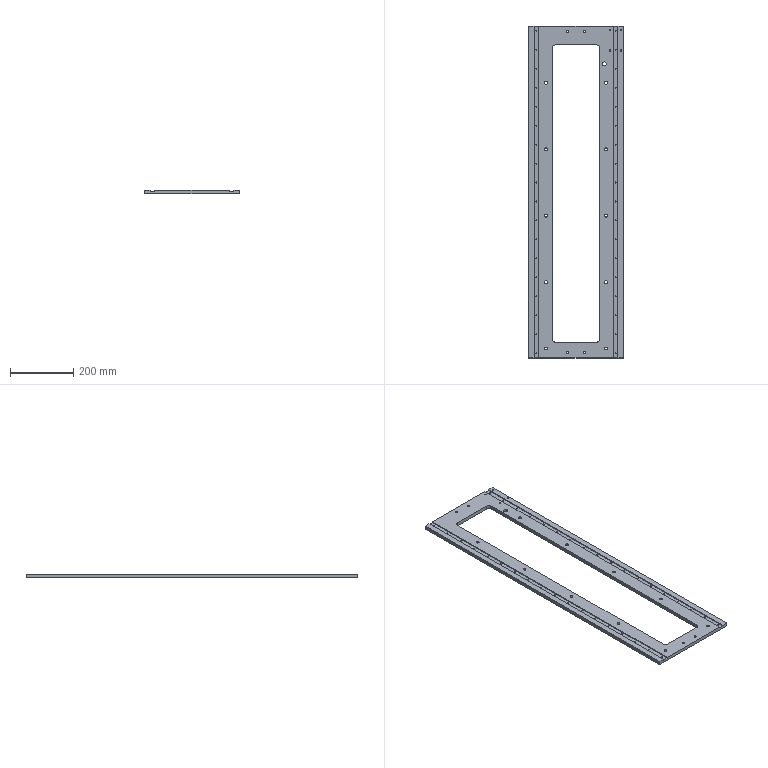Part | STEP file | X77-07001 | 1 solid | 204 faces | box 300 x 1050 x 12 mm | volume 1980727 mm3 | cylinder 114 | cone 72 | plane 18 | commonest cylinder face diameters 3.3 x72 9 x20 4.2 x8 6.8 x8 20 x4 12.5 x2